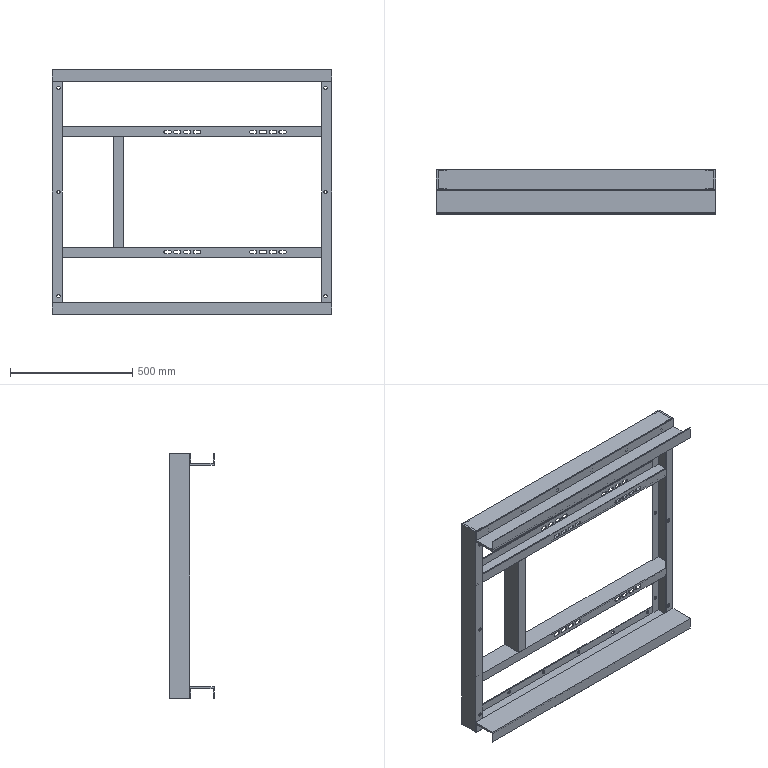Part | SolidWorks | 9 solids | 354 faces | box 1140 x 180 x 1000 mm | volume 8629233 mm3 | plane 186 | cylinder 168 | commonest cylinder face diameters 14 x168